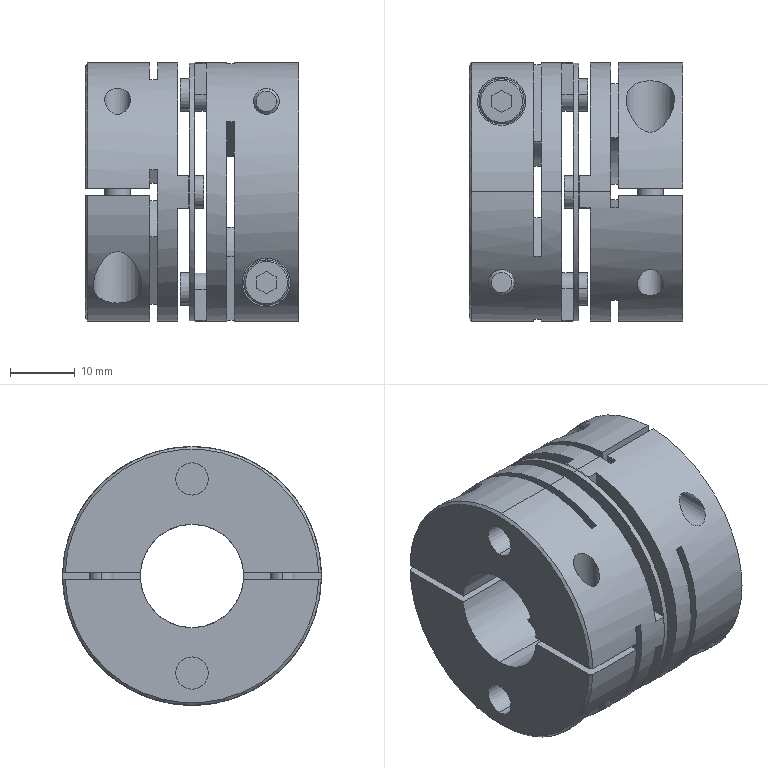Part | SolidWorks | features BaseBody 5 | 5 solids | 200 faces | box 33 x 40 x 40 mm | volume 24742 mm3 | plane 92 | cylinder 85 | cone 23 | commonest cylinder face diameters 5 x29 4 x24 7 x8 7.5 x8 40 x6 16 x4